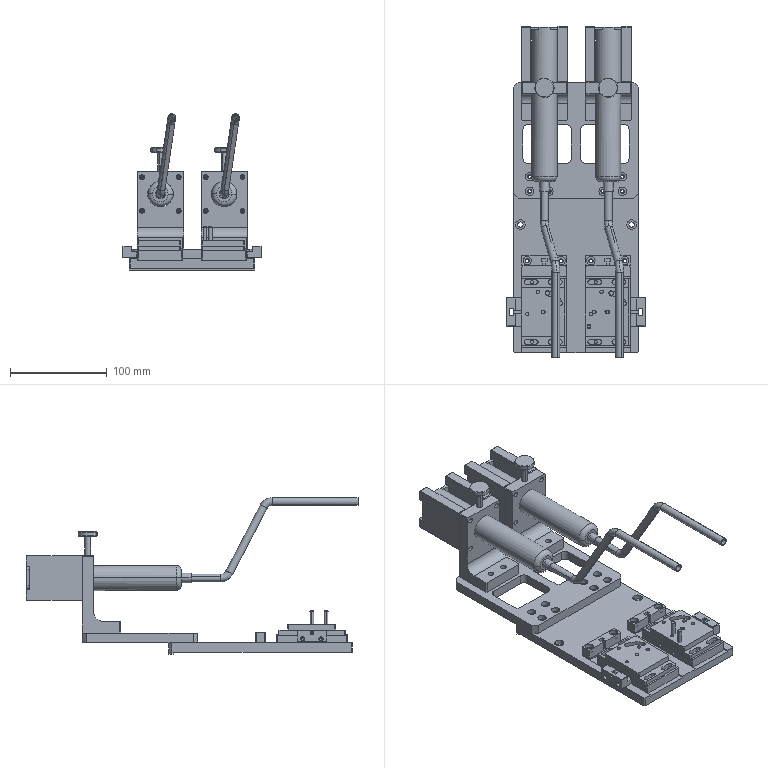Part | NX | features BREP 15 | 29 solids | 888 faces | box 143 x 343.823 x 162.131 mm | volume 750700 mm3 | cylinder 422 | plane 370 | cone 72 | torus 24 | commonest cylinder face diameters 3.3 x88 4.5 x80 6 x40 4 x32 8.6 x24 4.2 x20